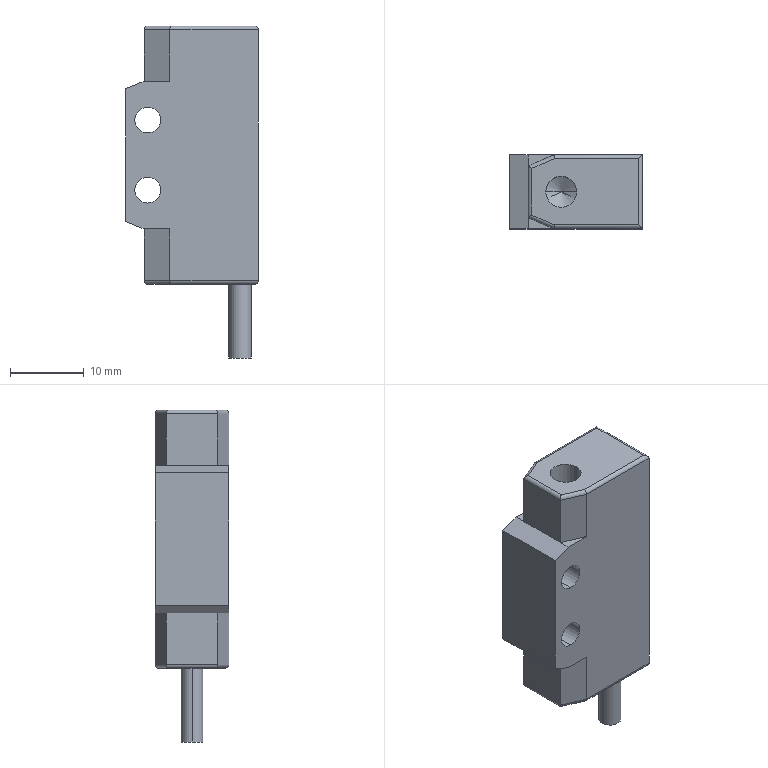Part | STEP file | 1 solid | 166 faces | box 18 x 10 x 45 mm | volume 5334 mm3 | plane 107 | spline 31 | cylinder 24 | cone 4 | commonest cylinder face diameters 1 x12 3.5 x4 4.2 x4 3 x2 0.875 x1 6.365 x1